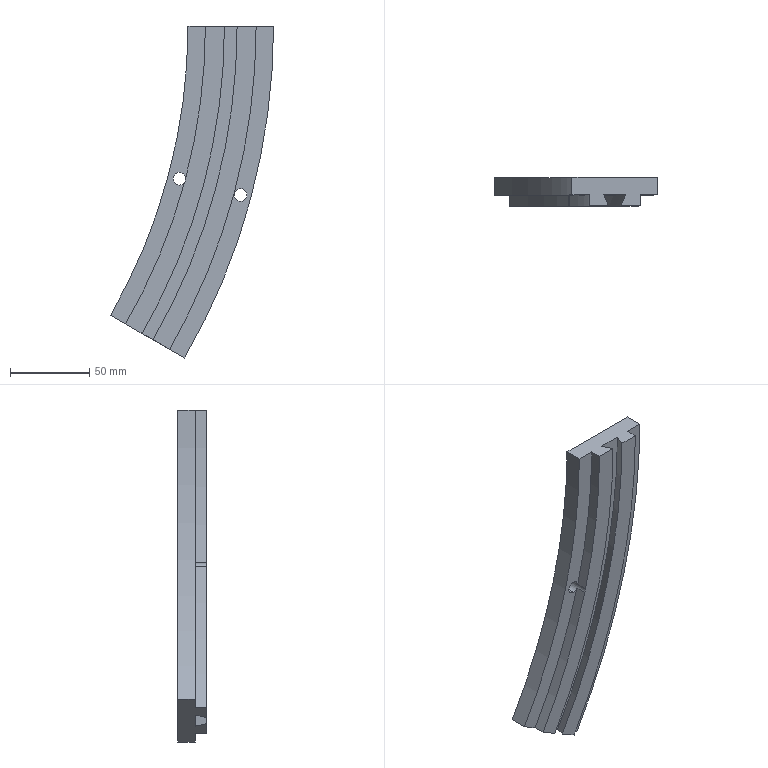Part | NX | features BREP 1 | 1 solid | 19 faces | box 102.901 x 18 x 209.5 mm | volume 150982 mm3 | cylinder 9 | plane 8 | cone 2 | commonest cylinder face diameters 8 x4 752 x2 730 x1 816 x1 838 x1
STEP:
#1=CARTESIAN_POINT('',(6.194,18.,-110.696));
#2=VERTEX_POINT('',#1);
#3=CARTESIAN_POINT('',(6.194,18.,-102.696));
#4=VERTEX_POINT('',#3);
#5=CARTESIAN_POINT('',(6.194,18.,-106.696));
#6=DIRECTION('',(0.,1.,0.));
#7=DIRECTION('',(0.,0.,1.));
#8=AXIS2_PLACEMENT_3D('',#5,#6,#7);
#9=CIRCLE('',#8,4.);
#10=EDGE_CURVE('',#2,#4,#9,.T.);
#11=ORIENTED_EDGE('',*,*,#10,.T.);
#12=CARTESIAN_POINT('',(6.194,7.,-102.696));
#13=VERTEX_POINT('',#12);
#14=CARTESIAN_POINT('',(6.194,18.001,-102.696));
#15=DIRECTION('',(0.,-1.,0.));
#16=VECTOR('',#15,1000.);
#17=LINE('',#14,#16);
#18=EDGE_CURVE('',#13,#4,#17,.F.);
#19=ORIENTED_EDGE('',*,*,#18,.F.);
#20=CARTESIAN_POINT('',(6.194,7.,-110.696));
#21=VERTEX_POINT('',#20);
#22=CARTESIAN_POINT('',(6.194,7.,-106.696));
#23=DIRECTION('',(0.,-1.,0.));
#24=DIRECTION('',(0.,0.,-1.));
#25=AXIS2_PLACEMENT_3D('',#22,#23,#24);
#26=CIRCLE('',#25,4.);
#27=EDGE_CURVE('',#13,#21,#26,.T.);
#28=ORIENTED_EDGE('',*,*,#27,.T.);
#29=CARTESIAN_POINT('',(6.194,18.001,-110.696));
#30=DIRECTION('',(0.,-1.,0.));
#31=VECTOR('',#30,1000.);
#32=LINE('',#29,#31);
#33=EDGE_CURVE('',#21,#2,#32,.F.);
#34=ORIENTED_EDGE('',*,*,#33,.T.);
#35=EDGE_LOOP('',(#11,#19,#28,#34));
#36=FACE_BOUND('',#35,.T.);
#37=CARTESIAN_POINT('',(6.194,18.001,-106.696));
#38=DIRECTION('',(0.,-1.,0.));
#39=DIRECTION('',(0.,0.,1.));
#40=AXIS2_PLACEMENT_3D('',#37,#38,#39);
#41=CYLINDRICAL_SURFACE('',#40,4.);
#42=ADVANCED_FACE('',(#36),#41,.F.);
#43=CARTESIAN_POINT('',(-32.443,18.,-100.343));
#44=VERTEX_POINT('',#43);
#45=CARTESIAN_POINT('',(-32.443,18.,-92.343));
#46=VERTEX_POINT('',#45);
#47=CARTESIAN_POINT('',(-32.443,18.,-96.343));
#48=DIRECTION('',(0.,1.,0.));
#49=DIRECTION('',(0.,0.,1.));
#50=AXIS2_PLACEMENT_3D('',#47,#48,#49);
#51=CIRCLE('',#50,4.);
#52=EDGE_CURVE('',#44,#46,#51,.T.);
#53=ORIENTED_EDGE('',*,*,#52,.T.);
#54=CARTESIAN_POINT('',(-32.443,7.,-92.343));
#55=VERTEX_POINT('',#54);
#56=CARTESIAN_POINT('',(-32.443,18.001,-92.343));
#57=DIRECTION('',(0.,-1.,0.));
#58=VECTOR('',#57,1000.);
#59=LINE('',#56,#58);
#60=EDGE_CURVE('',#55,#46,#59,.F.);
#61=ORIENTED_EDGE('',*,*,#60,.F.);
#62=CARTESIAN_POINT('',(-32.443,7.,-100.343));
#63=VERTEX_POINT('',#62);
#64=CARTESIAN_POINT('',(-32.443,7.,-96.343));
#65=DIRECTION('',(0.,-1.,0.));
#66=DIRECTION('',(0.,0.,-1.));
#67=AXIS2_PLACEMENT_3D('',#64,#65,#66);
#68=CIRCLE('',#67,4.);
#69=EDGE_CURVE('',#55,#63,#68,.T.);
#70=ORIENTED_EDGE('',*,*,#69,.T.);
#71=CARTESIAN_POINT('',(-32.443,18.001,-100.343));
#72=DIRECTION('',(0.,-1.,0.));
#73=VECTOR('',#72,1000.);
#74=LINE('',#71,#73);
#75=EDGE_CURVE('',#63,#44,#74,.F.);
#76=ORIENTED_EDGE('',*,*,#75,.T.);
#77=EDGE_LOOP('',(#53,#61,#70,#76));
#78=FACE_BOUND('',#77,.T.);
#79=CARTESIAN_POINT('',(-32.443,18.001,-96.343));
#80=DIRECTION('',(0.,-1.,0.));
#81=DIRECTION('',(0.,0.,1.));
#82=AXIS2_PLACEMENT_3D('',#79,#80,#81);
#83=CYLINDRICAL_SURFACE('',#82,4.);
#84=ADVANCED_FACE('',(#78),#83,.F.);
#85=CARTESIAN_POINT('',(-75.901,18.,-182.5));
#86=VERTEX_POINT('',#85);
#87=CARTESIAN_POINT('',(-27.,18.,0.));
#88=VERTEX_POINT('',#87);
#89=CARTESIAN_POINT('',(-392.,18.,0.));
#90=DIRECTION('',(0.,-1.,0.));
#91=DIRECTION('',(0.,0.,-1.));
#92=AXIS2_PLACEMENT_3D('',#89,#90,#91);
#93=CIRCLE('',#92,365.);
#94=EDGE_CURVE('',#86,#88,#93,.T.);
#95=ORIENTED_EDGE('',*,*,#94,.T.);
#96=CARTESIAN_POINT('',(27.,18.,0.));
#97=VERTEX_POINT('',#96);
#98=CARTESIAN_POINT('',(-27.,18.,0.));
#99=DIRECTION('',(-1.,0.,0.));
#100=VECTOR('',#99,1000.);
#101=LINE('',#98,#100);
#102=EDGE_CURVE('',#97,#88,#101,.T.);
#103=ORIENTED_EDGE('',*,*,#102,.F.);
#104=CARTESIAN_POINT('',(-29.135,18.,-209.5));
#105=VERTEX_POINT('',#104);
#106=CARTESIAN_POINT('',(-392.,18.,0.));
#107=DIRECTION('',(0.,-1.,0.));
#108=DIRECTION('',(0.,0.,-1.));
#109=AXIS2_PLACEMENT_3D('',#106,#107,#108);
#110=CIRCLE('',#109,419.);
#111=EDGE_CURVE('',#105,#97,#110,.T.);
#112=ORIENTED_EDGE('',*,*,#111,.F.);
#113=CARTESIAN_POINT('',(-75.901,18.,-182.5));
#114=DIRECTION('',(-0.866,0.,0.5));
#115=VECTOR('',#114,1000.);
#116=LINE('',#113,#115);
#117=EDGE_CURVE('',#105,#86,#116,.T.);
#118=ORIENTED_EDGE('',*,*,#117,.T.);
#119=EDGE_LOOP('',(#95,#103,#112,#118));
#120=FACE_BOUND('',#119,.T.);
#121=ORIENTED_EDGE('',*,*,#52,.F.);
#122=CARTESIAN_POINT('',(-32.443,18.,-96.343));
#123=DIRECTION('',(0.,1.,0.));
#124=DIRECTION('',(0.,0.,1.));
#125=AXIS2_PLACEMENT_3D('',#122,#123,#124);
#126=CIRCLE('',#125,4.);
#127=EDGE_CURVE('',#46,#44,#126,.T.);
#128=ORIENTED_EDGE('',*,*,#127,.F.);
#129=EDGE_LOOP('',(#121,#128));
#130=FACE_BOUND('',#129,.T.);
#131=ORIENTED_EDGE('',*,*,#10,.F.);
#132=CARTESIAN_POINT('',(6.194,18.,-106.696));
#133=DIRECTION('',(0.,1.,0.));
#134=DIRECTION('',(0.,0.,1.));
#135=AXIS2_PLACEMENT_3D('',#132,#133,#134);
#136=CIRCLE('',#135,4.);
#137=EDGE_CURVE('',#4,#2,#136,.T.);
#138=ORIENTED_EDGE('',*,*,#137,.F.);
#139=EDGE_LOOP('',(#131,#138));
#140=FACE_BOUND('',#139,.T.);
#141=CARTESIAN_POINT('',(-75.901,18.,-182.5));
#142=DIRECTION('',(0.,1.,0.));
#143=DIRECTION('',(-1.,0.,0.));
#144=AXIS2_PLACEMENT_3D('',#141,#142,#143);
#145=PLANE('',#144);
#146=ADVANCED_FACE('',(#120,#130,#140),#145,.T.);
#147=CARTESIAN_POINT('',(-29.135,7.,-209.5));
#148=VERTEX_POINT('',#147);
#149=CARTESIAN_POINT('',(27.,7.,0.));
#150=VERTEX_POINT('',#149);
#151=CARTESIAN_POINT('',(-392.,7.,0.));
#152=DIRECTION('',(0.,-1.,0.));
#153=DIRECTION('',(0.,0.,-1.));
#154=AXIS2_PLACEMENT_3D('',#151,#152,#153);
#155=CIRCLE('',#154,419.);
#156=EDGE_CURVE('',#148,#150,#155,.T.);
#157=ORIENTED_EDGE('',*,*,#156,.T.);
#158=CARTESIAN_POINT('',(16.,7.,0.));
#159=VERTEX_POINT('',#158);
#160=CARTESIAN_POINT('',(16.,7.,0.));
#161=DIRECTION('',(1.,0.,0.));
#162=VECTOR('',#161,1000.);
#163=LINE('',#160,#162);
#164=EDGE_CURVE('',#159,#150,#163,.T.);
#165=ORIENTED_EDGE('',*,*,#164,.F.);
#166=CARTESIAN_POINT('',(-38.662,7.,-204.));
#167=VERTEX_POINT('',#166);
#168=CARTESIAN_POINT('',(-392.,7.,0.));
#169=DIRECTION('',(0.,-1.,0.));
#170=DIRECTION('',(0.,0.,-1.));
#171=AXIS2_PLACEMENT_3D('',#168,#169,#170);
#172=CIRCLE('',#171,408.);
#173=EDGE_CURVE('',#167,#159,#172,.T.);
#174=ORIENTED_EDGE('',*,*,#173,.F.);
#175=CARTESIAN_POINT('',(-38.662,7.,-204.));
#176=DIRECTION('',(0.866,0.,-0.5));
#177=VECTOR('',#176,1000.);
#178=LINE('',#175,#177);
#179=EDGE_CURVE('',#167,#148,#178,.T.);
#180=ORIENTED_EDGE('',*,*,#179,.T.);
#181=EDGE_LOOP('',(#157,#165,#174,#180));
#182=FACE_BOUND('',#181,.T.);
#183=CARTESIAN_POINT('',(6.194,7.,-106.696));
#184=DIRECTION('',(0.,-1.,0.));
#185=DIRECTION('',(0.,0.,-1.));
#186=AXIS2_PLACEMENT_3D('',#183,#184,#185);
#187=CIRCLE('',#186,4.);
#188=EDGE_CURVE('',#21,#13,#187,.T.);
#189=ORIENTED_EDGE('',*,*,#188,.F.);
#190=ORIENTED_EDGE('',*,*,#27,.F.);
#191=EDGE_LOOP('',(#189,#190));
#192=FACE_BOUND('',#191,.T.);
#193=CARTESIAN_POINT('',(-38.662,7.,-204.));
#194=DIRECTION('',(0.,-1.,0.));
#195=DIRECTION('',(0.,0.,1.));
#196=AXIS2_PLACEMENT_3D('',#193,#194,#195);
#197=PLANE('',#196);
#198=ADVANCED_FACE('',(#182,#192),#197,.T.);
#199=CARTESIAN_POINT('',(-66.374,7.,-188.));
#200=VERTEX_POINT('',#199);
#201=CARTESIAN_POINT('',(-29.17,7.,-98.643));
#202=VERTEX_POINT('',#201);
#203=CARTESIAN_POINT('',(-392.,7.,0.));
#204=DIRECTION('',(0.,-1.,0.));
#205=DIRECTION('',(0.,0.,-1.));
#206=AXIS2_PLACEMENT_3D('',#203,#204,#205);
#207=CIRCLE('',#206,376.);
#208=EDGE_CURVE('',#200,#202,#207,.T.);
#209=ORIENTED_EDGE('',*,*,#208,.T.);
#210=CARTESIAN_POINT('',(-32.443,7.,-96.343));
#211=DIRECTION('',(0.,-1.,0.));
#212=DIRECTION('',(0.,0.,-1.));
#213=AXIS2_PLACEMENT_3D('',#210,#211,#212);
#214=CIRCLE('',#213,4.);
#215=EDGE_CURVE('',#63,#202,#214,.T.);
#216=ORIENTED_EDGE('',*,*,#215,.F.);
#217=ORIENTED_EDGE('',*,*,#69,.F.);
#218=CARTESIAN_POINT('',(-28.458,7.,-95.987));
#219=VERTEX_POINT('',#218);
#220=CARTESIAN_POINT('',(-32.443,7.,-96.343));
#221=DIRECTION('',(0.,-1.,0.));
#222=DIRECTION('',(0.,0.,-1.));
#223=AXIS2_PLACEMENT_3D('',#220,#221,#222);
#224=CIRCLE('',#223,4.);
#225=EDGE_CURVE('',#219,#55,#224,.T.);
#226=ORIENTED_EDGE('',*,*,#225,.F.);
#227=CARTESIAN_POINT('',(-16.,7.,0.));
#228=VERTEX_POINT('',#227);
#229=CARTESIAN_POINT('',(-392.,7.,0.));
#230=DIRECTION('',(0.,-1.,0.));
#231=DIRECTION('',(0.,0.,-1.));
#232=AXIS2_PLACEMENT_3D('',#229,#230,#231);
#233=CIRCLE('',#232,376.);
#234=EDGE_CURVE('',#219,#228,#233,.T.);
#235=ORIENTED_EDGE('',*,*,#234,.T.);
#236=CARTESIAN_POINT('',(-27.,7.,0.));
#237=VERTEX_POINT('',#236);
#238=CARTESIAN_POINT('',(-16.,7.,0.));
#239=DIRECTION('',(1.,0.,0.));
#240=VECTOR('',#239,1000.);
#241=LINE('',#238,#240);
#242=EDGE_CURVE('',#237,#228,#241,.T.);
#243=ORIENTED_EDGE('',*,*,#242,.F.);
#244=CARTESIAN_POINT('',(-75.901,7.,-182.5));
#245=VERTEX_POINT('',#244);
#246=CARTESIAN_POINT('',(-392.,7.,0.));
#247=DIRECTION('',(0.,-1.,0.));
#248=DIRECTION('',(0.,0.,-1.));
#249=AXIS2_PLACEMENT_3D('',#246,#247,#248);
#250=CIRCLE('',#249,365.);
#251=EDGE_CURVE('',#245,#237,#250,.T.);
#252=ORIENTED_EDGE('',*,*,#251,.F.);
#253=CARTESIAN_POINT('',(-66.374,7.,-188.));
#254=DIRECTION('',(0.866,0.,-0.5));
#255=VECTOR('',#254,1000.);
#256=LINE('',#253,#255);
#257=EDGE_CURVE('',#245,#200,#256,.T.);
#258=ORIENTED_EDGE('',*,*,#257,.T.);
#259=EDGE_LOOP('',(#209,#216,#217,#226,#235,#243,#252,#258));
#260=FACE_BOUND('',#259,.T.);
#261=CARTESIAN_POINT('',(-66.374,7.,-188.));
#262=DIRECTION('',(0.,-1.,0.));
#263=DIRECTION('',(0.,0.,1.));
#264=AXIS2_PLACEMENT_3D('',#261,#262,#263);
#265=PLANE('',#264);
#266=ADVANCED_FACE('',(#260),#265,.T.);
#267=ORIENTED_EDGE('',*,*,#234,.F.);
#268=CARTESIAN_POINT('',(-28.458,0.,-95.987));
#269=VERTEX_POINT('',#268);
#270=CARTESIAN_POINT('',(-28.458,3.5,-95.987));
#271=DIRECTION('',(0.,1.,0.));
#272=VECTOR('',#271,1000.);
#273=LINE('',#270,#272);
#274=EDGE_CURVE('',#269,#219,#273,.T.);
#275=ORIENTED_EDGE('',*,*,#274,.F.);
#276=CARTESIAN_POINT('',(-16.,0.,0.));
#277=VERTEX_POINT('',#276);
#278=CARTESIAN_POINT('',(-392.,0.,0.));
#279=DIRECTION('',(0.,-1.,0.));
#280=DIRECTION('',(0.,0.,-1.));
#281=AXIS2_PLACEMENT_3D('',#278,#279,#280);
#282=CIRCLE('',#281,376.);
#283=EDGE_CURVE('',#269,#277,#282,.T.);
#284=ORIENTED_EDGE('',*,*,#283,.T.);
#285=CARTESIAN_POINT('',(-16.,0.,0.));
#286=DIRECTION('',(0.,-1.,0.));
#287=VECTOR('',#286,1000.);
#288=LINE('',#285,#287);
#289=EDGE_CURVE('',#228,#277,#288,.T.);
#290=ORIENTED_EDGE('',*,*,#289,.F.);
#291=EDGE_LOOP('',(#267,#275,#284,#290));
#292=FACE_BOUND('',#291,.T.);
#293=CARTESIAN_POINT('',(-392.,0.,0.));
#294=DIRECTION('',(0.,-1.,0.));
#295=DIRECTION('',(0.,0.,1.));
#296=AXIS2_PLACEMENT_3D('',#293,#294,#295);
#297=CYLINDRICAL_SURFACE('',#296,376.);
#298=ADVANCED_FACE('',(#292),#297,.F.);
#299=CARTESIAN_POINT('',(-66.374,0.,-188.));
#300=VERTEX_POINT('',#299);
#301=CARTESIAN_POINT('',(-29.17,0.,-98.643));
#302=VERTEX_POINT('',#301);
#303=CARTESIAN_POINT('',(-392.,0.,0.));
#304=DIRECTION('',(0.,-1.,0.));
#305=DIRECTION('',(0.,0.,-1.));
#306=AXIS2_PLACEMENT_3D('',#303,#304,#305);
#307=CIRCLE('',#306,376.);
#308=EDGE_CURVE('',#300,#302,#307,.T.);
#309=ORIENTED_EDGE('',*,*,#308,.T.);
#310=CARTESIAN_POINT('',(-29.17,3.5,-98.643));
#311=DIRECTION('',(0.,-1.,0.));
#312=VECTOR('',#311,1000.);
#313=LINE('',#310,#312);
#314=EDGE_CURVE('',#202,#302,#313,.T.);
#315=ORIENTED_EDGE('',*,*,#314,.F.);
#316=ORIENTED_EDGE('',*,*,#208,.F.);
#317=CARTESIAN_POINT('',(-66.374,0.,-188.));
#318=DIRECTION('',(0.,-1.,0.));
#319=VECTOR('',#318,1000.);
#320=LINE('',#317,#319);
#321=EDGE_CURVE('',#200,#300,#320,.T.);
#322=ORIENTED_EDGE('',*,*,#321,.T.);
#323=EDGE_LOOP('',(#309,#315,#316,#322));
#324=FACE_BOUND('',#323,.T.);
#325=CARTESIAN_POINT('',(-392.,0.,0.));
#326=DIRECTION('',(0.,-1.,0.));
#327=DIRECTION('',(0.,0.,1.));
#328=AXIS2_PLACEMENT_3D('',#325,#326,#327);
#329=CYLINDRICAL_SURFACE('',#328,376.);
#330=ADVANCED_FACE('',(#324),#329,.F.);
#331=ORIENTED_EDGE('',*,*,#283,.F.);
#332=CARTESIAN_POINT('',(-32.443,0.,-96.343));
#333=DIRECTION('',(0.,1.,0.));
#334=DIRECTION('',(0.,0.,1.));
#335=AXIS2_PLACEMENT_3D('',#332,#333,#334);
#336=CIRCLE('',#335,4.);
#337=EDGE_CURVE('',#269,#302,#336,.T.);
#338=ORIENTED_EDGE('',*,*,#337,.T.);
#339=ORIENTED_EDGE('',*,*,#308,.F.);
#340=CARTESIAN_POINT('',(-55.982,0.,-194.));
#341=VERTEX_POINT('',#340);
#342=CARTESIAN_POINT('',(-55.982,0.,-194.));
#343=DIRECTION('',(0.866,0.,-0.5));
#344=VECTOR('',#343,1000.);
#345=LINE('',#342,#344);
#346=EDGE_CURVE('',#300,#341,#345,.T.);
#347=ORIENTED_EDGE('',*,*,#346,.T.);
#348=CARTESIAN_POINT('',(-4.,0.,0.));
#349=VERTEX_POINT('',#348);
#350=CARTESIAN_POINT('',(-392.,0.,0.));
#351=DIRECTION('',(0.,-1.,0.));
#352=DIRECTION('',(0.,0.,-1.));
#353=AXIS2_PLACEMENT_3D('',#350,#351,#352);
#354=CIRCLE('',#353,388.);
#355=EDGE_CURVE('',#341,#349,#354,.T.);
#356=ORIENTED_EDGE('',*,*,#355,.T.);
#357=CARTESIAN_POINT('',(-4.,0.,0.));
#358=DIRECTION('',(1.,0.,0.));
#359=VECTOR('',#358,1000.);
#360=LINE('',#357,#359);
#361=EDGE_CURVE('',#277,#349,#360,.T.);
#362=ORIENTED_EDGE('',*,*,#361,.F.);
#363=EDGE_LOOP('',(#331,#338,#339,#347,#356,#362));
#364=FACE_BOUND('',#363,.T.);
#365=CARTESIAN_POINT('',(-55.982,0.,-194.));
#366=DIRECTION('',(0.,-1.,0.));
#367=DIRECTION('',(0.,0.,1.));
#368=AXIS2_PLACEMENT_3D('',#365,#366,#367);
#369=PLANE('',#368);
#370=ADVANCED_FACE('',(#364),#369,.T.);
#371=CARTESIAN_POINT('',(-38.662,0.,-204.));
#372=VERTEX_POINT('',#371);
#373=CARTESIAN_POINT('',(16.,0.,0.));
#374=VERTEX_POINT('',#373);
#375=CARTESIAN_POINT('',(-392.,0.,0.));
#376=DIRECTION('',(0.,-1.,0.));
#377=DIRECTION('',(0.,0.,-1.));
#378=AXIS2_PLACEMENT_3D('',#375,#376,#377);
#379=CIRCLE('',#378,408.);
#380=EDGE_CURVE('',#372,#374,#379,.T.);
#381=ORIENTED_EDGE('',*,*,#380,.T.);
#382=CARTESIAN_POINT('',(4.,0.,0.));
#383=VERTEX_POINT('',#382);
#384=CARTESIAN_POINT('',(4.,0.,0.));
#385=DIRECTION('',(1.,0.,0.));
#386=VECTOR('',#385,1000.);
#387=LINE('',#384,#386);
#388=EDGE_CURVE('',#383,#374,#387,.T.);
#389=ORIENTED_EDGE('',*,*,#388,.F.);
#390=CARTESIAN_POINT('',(-49.054,0.,-198.));
#391=VERTEX_POINT('',#390);
#392=CARTESIAN_POINT('',(-392.,0.,0.));
#393=DIRECTION('',(0.,-1.,0.));
#394=DIRECTION('',(0.,0.,-1.));
#395=AXIS2_PLACEMENT_3D('',#392,#393,#394);
#396=CIRCLE('',#395,396.);
#397=EDGE_CURVE('',#391,#383,#396,.T.);
#398=ORIENTED_EDGE('',*,*,#397,.F.);
#399=CARTESIAN_POINT('',(-49.054,0.,-198.));
#400=DIRECTION('',(0.866,0.,-0.5));
#401=VECTOR('',#400,1000.);
#402=LINE('',#399,#401);
#403=EDGE_CURVE('',#391,#372,#402,.T.);
#404=ORIENTED_EDGE('',*,*,#403,.T.);
#405=EDGE_LOOP('',(#381,#389,#398,#404));
#406=FACE_BOUND('',#405,.T.);
#407=CARTESIAN_POINT('',(-49.054,0.,-198.));
#408=DIRECTION('',(0.,-1.,0.));
#409=DIRECTION('',(0.,0.,1.));
#410=AXIS2_PLACEMENT_3D('',#407,#408,#409);
#411=PLANE('',#410);
#412=ADVANCED_FACE('',(#406),#411,.T.);
#413=ORIENTED_EDGE('',*,*,#173,.T.);
#414=CARTESIAN_POINT('',(16.,0.,0.));
#415=DIRECTION('',(0.,1.,0.));
#416=VECTOR('',#415,1000.);
#417=LINE('',#414,#416);
#418=EDGE_CURVE('',#374,#159,#417,.T.);
#419=ORIENTED_EDGE('',*,*,#418,.F.);
#420=ORIENTED_EDGE('',*,*,#380,.F.);
#421=CARTESIAN_POINT('',(-38.662,0.,-204.));
#422=DIRECTION('',(0.,1.,0.));
#423=VECTOR('',#422,1000.);
#424=LINE('',#421,#423);
#425=EDGE_CURVE('',#372,#167,#424,.T.);
#426=ORIENTED_EDGE('',*,*,#425,.T.);
#427=EDGE_LOOP('',(#413,#419,#420,#426));
#428=FACE_BOUND('',#427,.T.);
#429=CARTESIAN_POINT('',(-392.,0.,0.));
#430=DIRECTION('',(0.,-1.,0.));
#431=DIRECTION('',(0.,0.,1.));
#432=AXIS2_PLACEMENT_3D('',#429,#430,#431);
#433=CYLINDRICAL_SURFACE('',#432,408.);
#434=ADVANCED_FACE('',(#428),#433,.T.);
#435=ORIENTED_EDGE('',*,*,#111,.T.);
#436=CARTESIAN_POINT('',(27.,7.,0.));
#437=DIRECTION('',(0.,1.,0.));
#438=VECTOR('',#437,1000.);
#439=LINE('',#436,#438);
#440=EDGE_CURVE('',#150,#97,#439,.T.);
#441=ORIENTED_EDGE('',*,*,#440,.F.);
#442=ORIENTED_EDGE('',*,*,#156,.F.);
#443=CARTESIAN_POINT('',(-29.135,7.,-209.5));
#444=DIRECTION('',(0.,1.,0.));
#445=VECTOR('',#444,1000.);
#446=LINE('',#443,#445);
#447=EDGE_CURVE('',#148,#105,#446,.T.);
#448=ORIENTED_EDGE('',*,*,#447,.T.);
#449=EDGE_LOOP('',(#435,#441,#442,#448));
#450=FACE_BOUND('',#449,.T.);
#451=CARTESIAN_POINT('',(-392.,0.,0.));
#452=DIRECTION('',(0.,-1.,0.));
#453=DIRECTION('',(0.,0.,1.));
#454=AXIS2_PLACEMENT_3D('',#451,#452,#453);
#455=CYLINDRICAL_SURFACE('',#454,419.);
#456=ADVANCED_FACE('',(#450),#455,.T.);
#457=ORIENTED_EDGE('',*,*,#251,.T.);
#458=CARTESIAN_POINT('',(-27.,7.,0.));
#459=DIRECTION('',(0.,-1.,0.));
#460=VECTOR('',#459,1000.);
#461=LINE('',#458,#460);
#462=EDGE_CURVE('',#88,#237,#461,.T.);
#463=ORIENTED_EDGE('',*,*,#462,.F.);
#464=ORIENTED_EDGE('',*,*,#94,.F.);
#465=CARTESIAN_POINT('',(-75.901,7.,-182.5));
#466=DIRECTION('',(0.,-1.,0.));
#467=VECTOR('',#466,1000.);
#468=LINE('',#465,#467);
#469=EDGE_CURVE('',#86,#245,#468,.T.);
#470=ORIENTED_EDGE('',*,*,#469,.T.);
#471=EDGE_LOOP('',(#457,#463,#464,#470));
#472=FACE_BOUND('',#471,.T.);
#473=CARTESIAN_POINT('',(-392.,0.,0.));
#474=DIRECTION('',(0.,-1.,0.));
#475=DIRECTION('',(0.,0.,1.));
#476=AXIS2_PLACEMENT_3D('',#473,#474,#475);
#477=CYLINDRICAL_SURFACE('',#476,365.);
#478=ADVANCED_FACE('',(#472),#477,.F.);
#479=CARTESIAN_POINT('',(-58.58,7.,-192.5));
#480=VERTEX_POINT('',#479);
#481=CARTESIAN_POINT('',(-7.,7.,0.));
#482=VERTEX_POINT('',#481);
#483=CARTESIAN_POINT('',(-392.,7.,0.));
#484=DIRECTION('',(0.,-1.,0.));
#485=DIRECTION('',(0.,0.,-1.));
#486=AXIS2_PLACEMENT_3D('',#483,#484,#485);
#487=CIRCLE('',#486,385.);
#488=EDGE_CURVE('',#480,#482,#487,.T.);
#489=ORIENTED_EDGE('',*,*,#488,.T.);
#490=CARTESIAN_POINT('',(-7.,7.,0.));
#491=DIRECTION('',(-0.3939,0.9191,0.));
#492=VECTOR('',#491,1000.);
#493=LINE('',#490,#492);
#494=EDGE_CURVE('',#349,#482,#493,.T.);
#495=ORIENTED_EDGE('',*,*,#494,.F.);
#496=ORIENTED_EDGE('',*,*,#355,.F.);
#497=CARTESIAN_POINT('',(-58.58,7.,-192.5));
#498=DIRECTION('',(-0.3411,0.9191,0.197));
#499=VECTOR('',#498,1000.);
#500=LINE('',#497,#499);
#501=EDGE_CURVE('',#341,#480,#500,.T.);
#502=ORIENTED_EDGE('',*,*,#501,.T.);
#503=EDGE_LOOP('',(#489,#495,#496,#502));
#504=FACE_BOUND('',#503,.T.);
#505=CARTESIAN_POINT('',(-392.,0.,0.));
#506=DIRECTION('',(0.,-1.,0.));
#507=DIRECTION('',(0.,0.,1.));
#508=AXIS2_PLACEMENT_3D('',#505,#506,#507);
#509=CONICAL_SURFACE('',#508,388.,0.4049);
#510=ADVANCED_FACE('',(#504),#509,.T.);
#511=CARTESIAN_POINT('',(-46.456,7.,-199.5));
#512=VERTEX_POINT('',#511);
#513=CARTESIAN_POINT('',(7.,7.,0.));
#514=VERTEX_POINT('',#513);
#515=CARTESIAN_POINT('',(-392.,7.,0.));
#516=DIRECTION('',(0.,-1.,0.));
#517=DIRECTION('',(0.,0.,-1.));
#518=AXIS2_PLACEMENT_3D('',#515,#516,#517);
#519=CIRCLE('',#518,399.);
#520=EDGE_CURVE('',#512,#514,#519,.T.);
#521=ORIENTED_EDGE('',*,*,#520,.T.);
#522=CARTESIAN_POINT('',(7.,7.,0.));
#523=DIRECTION('',(1.,0.,0.));
#524=VECTOR('',#523,1000.);
#525=LINE('',#522,#524);
#526=EDGE_CURVE('',#482,#514,#525,.T.);
#527=ORIENTED_EDGE('',*,*,#526,.F.);
#528=ORIENTED_EDGE('',*,*,#488,.F.);
#529=CARTESIAN_POINT('',(-46.456,7.,-199.5));
#530=DIRECTION('',(0.866,0.,-0.5));
#531=VECTOR('',#530,1000.);
#532=LINE('',#529,#531);
#533=EDGE_CURVE('',#480,#512,#532,.T.);
#534=ORIENTED_EDGE('',*,*,#533,.T.);
#535=EDGE_LOOP('',(#521,#527,#528,#534));
#536=FACE_BOUND('',#535,.T.);
#537=CARTESIAN_POINT('',(-46.456,7.,-199.5));
#538=DIRECTION('',(0.,-1.,0.));
#539=DIRECTION('',(0.,0.,1.));
#540=AXIS2_PLACEMENT_3D('',#537,#538,#539);
#541=PLANE('',#540);
#542=ADVANCED_FACE('',(#536),#541,.T.);
#543=CARTESIAN_POINT('',(-46.456,7.,-199.5));
#544=DIRECTION('',(-0.3411,-0.9191,0.197));
#545=VECTOR('',#544,1000.);
#546=LINE('',#543,#545);
#547=EDGE_CURVE('',#512,#391,#546,.T.);
#548=ORIENTED_EDGE('',*,*,#547,.T.);
#549=ORIENTED_EDGE('',*,*,#397,.T.);
#550=CARTESIAN_POINT('',(7.,7.,0.));
#551=DIRECTION('',(-0.3939,-0.9191,0.));
#552=VECTOR('',#551,1000.);
#553=LINE('',#550,#552);
#554=EDGE_CURVE('',#514,#383,#553,.T.);
#555=ORIENTED_EDGE('',*,*,#554,.F.);
#556=ORIENTED_EDGE('',*,*,#520,.F.);
#557=EDGE_LOOP('',(#548,#549,#555,#556));
#558=FACE_BOUND('',#557,.T.);
#559=CARTESIAN_POINT('',(-392.,7.,0.));
#560=DIRECTION('',(0.,1.,0.));
#561=DIRECTION('',(0.,0.,-1.));
#562=AXIS2_PLACEMENT_3D('',#559,#560,#561);
#563=CONICAL_SURFACE('',#562,399.,0.4049);
#564=ADVANCED_FACE('',(#558),#563,.F.);
#565=ORIENTED_EDGE('',*,*,#403,.F.);
#566=ORIENTED_EDGE('',*,*,#547,.F.);
#567=ORIENTED_EDGE('',*,*,#533,.F.);
#568=ORIENTED_EDGE('',*,*,#501,.F.);
#569=ORIENTED_EDGE('',*,*,#346,.F.);
#570=ORIENTED_EDGE('',*,*,#321,.F.);
#571=ORIENTED_EDGE('',*,*,#257,.F.);
#572=ORIENTED_EDGE('',*,*,#469,.F.);
#573=ORIENTED_EDGE('',*,*,#117,.F.);
#574=ORIENTED_EDGE('',*,*,#447,.F.);
#575=ORIENTED_EDGE('',*,*,#179,.F.);
#576=ORIENTED_EDGE('',*,*,#425,.F.);
#577=EDGE_LOOP('',(#565,#566,#567,#568,#569,#570,#571,#572,#573,#574,#575,#576));
#578=FACE_BOUND('',#577,.T.);
#579=CARTESIAN_POINT('',(-52.518,0.,-196.));
#580=DIRECTION('',(0.5,0.,0.866));
#581=DIRECTION('',(0.,1.,0.));
#582=AXIS2_PLACEMENT_3D('',#579,#580,#581);
#583=PLANE('',#582);
#584=ADVANCED_FACE('',(#578),#583,.F.);
#585=ORIENTED_EDGE('',*,*,#388,.T.);
#586=ORIENTED_EDGE('',*,*,#418,.T.);
#587=ORIENTED_EDGE('',*,*,#164,.T.);
#588=ORIENTED_EDGE('',*,*,#440,.T.);
#589=ORIENTED_EDGE('',*,*,#102,.T.);
#590=ORIENTED_EDGE('',*,*,#462,.T.);
#591=ORIENTED_EDGE('',*,*,#242,.T.);
#592=ORIENTED_EDGE('',*,*,#289,.T.);
#593=ORIENTED_EDGE('',*,*,#361,.T.);
#594=ORIENTED_EDGE('',*,*,#494,.T.);
#595=ORIENTED_EDGE('',*,*,#526,.T.);
#596=ORIENTED_EDGE('',*,*,#554,.T.);
#597=EDGE_LOOP('',(#585,#586,#587,#588,#589,#590,#591,#592,#593,#594,#595,#596));
#598=FACE_BOUND('',#597,.T.);
#599=CARTESIAN_POINT('',(0.,0.,0.));
#600=DIRECTION('',(0.,0.,1.));
#601=DIRECTION('',(-1.,0.,0.));
#602=AXIS2_PLACEMENT_3D('',#599,#600,#601);
#603=PLANE('',#602);
#604=ADVANCED_FACE('',(#598),#603,.T.);
#605=ORIENTED_EDGE('',*,*,#60,.T.);
#606=ORIENTED_EDGE('',*,*,#127,.T.);
#607=ORIENTED_EDGE('',*,*,#75,.F.);
#608=ORIENTED_EDGE('',*,*,#215,.T.);
#609=ORIENTED_EDGE('',*,*,#314,.T.);
#610=ORIENTED_EDGE('',*,*,#337,.F.);
#611=ORIENTED_EDGE('',*,*,#274,.T.);
#612=ORIENTED_EDGE('',*,*,#225,.T.);
#613=EDGE_LOOP('',(#605,#606,#607,#608,#609,#610,#611,#612));
#614=FACE_BOUND('',#613,.T.);
#615=CARTESIAN_POINT('',(-32.443,18.001,-96.343));
#616=DIRECTION('',(0.,-1.,0.));
#617=DIRECTION('',(0.,0.,1.));
#618=AXIS2_PLACEMENT_3D('',#615,#616,#617);
#619=CYLINDRICAL_SURFACE('',#618,4.);
#620=ADVANCED_FACE('',(#614),#619,.F.);
#621=ORIENTED_EDGE('',*,*,#18,.T.);
#622=ORIENTED_EDGE('',*,*,#137,.T.);
#623=ORIENTED_EDGE('',*,*,#33,.F.);
#624=ORIENTED_EDGE('',*,*,#188,.T.);
#625=EDGE_LOOP('',(#621,#622,#623,#624));
#626=FACE_BOUND('',#625,.T.);
#627=CARTESIAN_POINT('',(6.194,18.001,-106.696));
#628=DIRECTION('',(0.,-1.,0.));
#629=DIRECTION('',(0.,0.,1.));
#630=AXIS2_PLACEMENT_3D('',#627,#628,#629);
#631=CYLINDRICAL_SURFACE('',#630,4.);
#632=ADVANCED_FACE('',(#626),#631,.F.);
#633=CLOSED_SHELL('',(#42,#84,#146,#198,#266,#298,#330,#370,#412,#434,#456,#478,#510,#542,#564,#584,#604,#620,#632));
#634=MANIFOLD_SOLID_BREP('',#633);
#635=(LENGTH_UNIT()NAMED_UNIT(*)SI_UNIT(.MILLI.,.METRE.));
#636=UNCERTAINTY_MEASURE_WITH_UNIT(LENGTH_MEASURE(0.00001),#635,'','');
#637=(NAMED_UNIT(*)PLANE_ANGLE_UNIT()SI_UNIT($,.RADIAN.));
#638=(NAMED_UNIT(*)SI_UNIT($,.STERADIAN.)SOLID_ANGLE_UNIT());
#639=(GEOMETRIC_REPRESENTATION_CONTEXT(3)GLOBAL_UNCERTAINTY_ASSIGNED_CONTEXT((#636))GLOBAL_UNIT_ASSIGNED_CONTEXT((#635,#637,#638))REPRESENTATION_CONTEXT('',''));
#640=ADVANCED_BREP_SHAPE_REPRESENTATION('',(#634),#639);